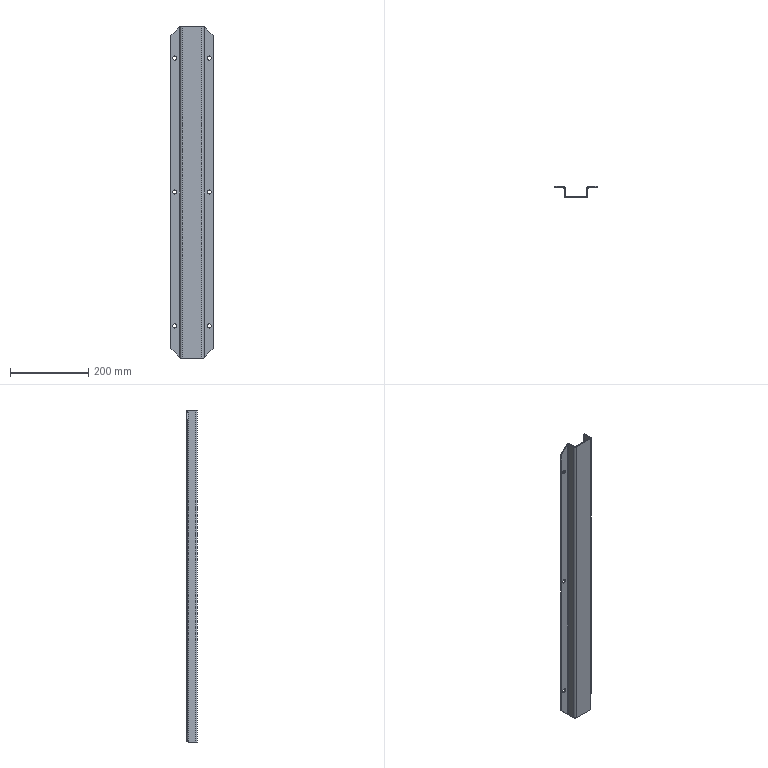Part | STEP file | 750078193 | 1 solid | 42 faces | box 108 x 27.5 x 850 mm | volume 319697 mm3 | cylinder 20 | plane 18 | spline 4 | commonest cylinder face diameters 10.5 x12 4 x4 9 x4
STEP:
#1=CARTESIAN_POINT('',(44.,27.5,-5.25));
#2=VERTEX_POINT('',#1);
#3=CARTESIAN_POINT('',(44.,27.5,5.25));
#4=VERTEX_POINT('',#3);
#5=CARTESIAN_POINT('',(44.,27.5,0.));
#6=DIRECTION('',(0.,1.,0.));
#7=DIRECTION('',(0.,0.,-1.));
#8=AXIS2_PLACEMENT_3D('',#5,#6,#7);
#9=CIRCLE('',#8,5.25);
#10=EDGE_CURVE('',#2,#4,#9,.T.);
#11=ORIENTED_EDGE('',*,*,#10,.T.);
#12=CARTESIAN_POINT('',(44.,25.,5.25));
#13=VERTEX_POINT('',#12);
#14=CARTESIAN_POINT('',(44.,882.275,5.25));
#15=DIRECTION('',(0.,-1.,0.));
#16=VECTOR('',#15,1000.);
#17=LINE('',#14,#16);
#18=EDGE_CURVE('',#4,#13,#17,.T.);
#19=ORIENTED_EDGE('',*,*,#18,.T.);
#20=CARTESIAN_POINT('',(44.,25.,-5.25));
#21=VERTEX_POINT('',#20);
#22=CARTESIAN_POINT('',(44.,25.,0.));
#23=DIRECTION('',(0.,1.,0.));
#24=DIRECTION('',(0.,0.,-1.));
#25=AXIS2_PLACEMENT_3D('',#22,#23,#24);
#26=CIRCLE('',#25,5.25);
#27=EDGE_CURVE('',#21,#13,#26,.T.);
#28=ORIENTED_EDGE('',*,*,#27,.F.);
#29=CARTESIAN_POINT('',(44.,882.275,-5.25));
#30=DIRECTION('',(0.,-1.,0.));
#31=VECTOR('',#30,1000.);
#32=LINE('',#29,#31);
#33=EDGE_CURVE('',#2,#21,#32,.T.);
#34=ORIENTED_EDGE('',*,*,#33,.F.);
#35=EDGE_LOOP('',(#11,#19,#28,#34));
#36=FACE_OUTER_BOUND('',#35,.T.);
#37=CARTESIAN_POINT('',(44.,882.275,0.));
#38=DIRECTION('',(0.,-1.,0.));
#39=DIRECTION('',(0.,0.,-1.));
#40=AXIS2_PLACEMENT_3D('',#37,#38,#39);
#41=CYLINDRICAL_SURFACE('',#40,5.25);
#42=ADVANCED_FACE('',(#36),#41,.F.);
#43=CARTESIAN_POINT('',(44.,27.5,-348.25));
#44=VERTEX_POINT('',#43);
#45=CARTESIAN_POINT('',(44.,27.5,-337.75));
#46=VERTEX_POINT('',#45);
#47=CARTESIAN_POINT('',(44.,27.5,-343.));
#48=DIRECTION('',(0.,1.,0.));
#49=DIRECTION('',(0.,0.,-1.));
#50=AXIS2_PLACEMENT_3D('',#47,#48,#49);
#51=CIRCLE('',#50,5.25);
#52=EDGE_CURVE('',#44,#46,#51,.T.);
#53=ORIENTED_EDGE('',*,*,#52,.T.);
#54=CARTESIAN_POINT('',(44.,25.,-337.75));
#55=VERTEX_POINT('',#54);
#56=CARTESIAN_POINT('',(44.,882.275,-337.75));
#57=DIRECTION('',(0.,-1.,0.));
#58=VECTOR('',#57,1000.);
#59=LINE('',#56,#58);
#60=EDGE_CURVE('',#46,#55,#59,.T.);
#61=ORIENTED_EDGE('',*,*,#60,.T.);
#62=CARTESIAN_POINT('',(44.,25.,-348.25));
#63=VERTEX_POINT('',#62);
#64=CARTESIAN_POINT('',(44.,25.,-343.));
#65=DIRECTION('',(0.,1.,0.));
#66=DIRECTION('',(0.,0.,-1.));
#67=AXIS2_PLACEMENT_3D('',#64,#65,#66);
#68=CIRCLE('',#67,5.25);
#69=EDGE_CURVE('',#63,#55,#68,.T.);
#70=ORIENTED_EDGE('',*,*,#69,.F.);
#71=CARTESIAN_POINT('',(44.,882.275,-348.25));
#72=DIRECTION('',(0.,-1.,0.));
#73=VECTOR('',#72,1000.);
#74=LINE('',#71,#73);
#75=EDGE_CURVE('',#44,#63,#74,.T.);
#76=ORIENTED_EDGE('',*,*,#75,.F.);
#77=EDGE_LOOP('',(#53,#61,#70,#76));
#78=FACE_OUTER_BOUND('',#77,.T.);
#79=CARTESIAN_POINT('',(44.,882.275,-343.));
#80=DIRECTION('',(0.,-1.,0.));
#81=DIRECTION('',(0.,0.,-1.));
#82=AXIS2_PLACEMENT_3D('',#79,#80,#81);
#83=CYLINDRICAL_SURFACE('',#82,5.25);
#84=ADVANCED_FACE('',(#78),#83,.F.);
#85=CARTESIAN_POINT('',(44.,27.5,337.75));
#86=VERTEX_POINT('',#85);
#87=CARTESIAN_POINT('',(44.,27.5,348.25));
#88=VERTEX_POINT('',#87);
#89=CARTESIAN_POINT('',(44.,27.5,343.));
#90=DIRECTION('',(0.,1.,0.));
#91=DIRECTION('',(0.,0.,-1.));
#92=AXIS2_PLACEMENT_3D('',#89,#90,#91);
#93=CIRCLE('',#92,5.25);
#94=EDGE_CURVE('',#86,#88,#93,.T.);
#95=ORIENTED_EDGE('',*,*,#94,.T.);
#96=CARTESIAN_POINT('',(44.,25.,348.25));
#97=VERTEX_POINT('',#96);
#98=CARTESIAN_POINT('',(44.,882.275,348.25));
#99=DIRECTION('',(0.,-1.,0.));
#100=VECTOR('',#99,1000.);
#101=LINE('',#98,#100);
#102=EDGE_CURVE('',#88,#97,#101,.T.);
#103=ORIENTED_EDGE('',*,*,#102,.T.);
#104=CARTESIAN_POINT('',(44.,25.,337.75));
#105=VERTEX_POINT('',#104);
#106=CARTESIAN_POINT('',(44.,25.,343.));
#107=DIRECTION('',(0.,1.,0.));
#108=DIRECTION('',(0.,0.,-1.));
#109=AXIS2_PLACEMENT_3D('',#106,#107,#108);
#110=CIRCLE('',#109,5.25);
#111=EDGE_CURVE('',#105,#97,#110,.T.);
#112=ORIENTED_EDGE('',*,*,#111,.F.);
#113=CARTESIAN_POINT('',(44.,882.275,337.75));
#114=DIRECTION('',(0.,-1.,0.));
#115=VECTOR('',#114,1000.);
#116=LINE('',#113,#115);
#117=EDGE_CURVE('',#86,#105,#116,.T.);
#118=ORIENTED_EDGE('',*,*,#117,.F.);
#119=EDGE_LOOP('',(#95,#103,#112,#118));
#120=FACE_OUTER_BOUND('',#119,.T.);
#121=CARTESIAN_POINT('',(44.,882.275,343.));
#122=DIRECTION('',(0.,-1.,0.));
#123=DIRECTION('',(0.,0.,-1.));
#124=AXIS2_PLACEMENT_3D('',#121,#122,#123);
#125=CYLINDRICAL_SURFACE('',#124,5.25);
#126=ADVANCED_FACE('',(#120),#125,.F.);
#127=CARTESIAN_POINT('',(-44.,27.5,337.75));
#128=VERTEX_POINT('',#127);
#129=CARTESIAN_POINT('',(-44.,27.5,348.25));
#130=VERTEX_POINT('',#129);
#131=CARTESIAN_POINT('',(-44.,27.5,343.));
#132=DIRECTION('',(0.,1.,0.));
#133=DIRECTION('',(0.,0.,-1.));
#134=AXIS2_PLACEMENT_3D('',#131,#132,#133);
#135=CIRCLE('',#134,5.25);
#136=EDGE_CURVE('',#128,#130,#135,.T.);
#137=ORIENTED_EDGE('',*,*,#136,.T.);
#138=CARTESIAN_POINT('',(-44.,25.,348.25));
#139=VERTEX_POINT('',#138);
#140=CARTESIAN_POINT('',(-44.,882.275,348.25));
#141=DIRECTION('',(0.,-1.,0.));
#142=VECTOR('',#141,1000.);
#143=LINE('',#140,#142);
#144=EDGE_CURVE('',#130,#139,#143,.T.);
#145=ORIENTED_EDGE('',*,*,#144,.T.);
#146=CARTESIAN_POINT('',(-44.,25.,337.75));
#147=VERTEX_POINT('',#146);
#148=CARTESIAN_POINT('',(-44.,25.,343.));
#149=DIRECTION('',(0.,1.,0.));
#150=DIRECTION('',(0.,0.,-1.));
#151=AXIS2_PLACEMENT_3D('',#148,#149,#150);
#152=CIRCLE('',#151,5.25);
#153=EDGE_CURVE('',#147,#139,#152,.T.);
#154=ORIENTED_EDGE('',*,*,#153,.F.);
#155=CARTESIAN_POINT('',(-44.,882.275,337.75));
#156=DIRECTION('',(0.,-1.,0.));
#157=VECTOR('',#156,1000.);
#158=LINE('',#155,#157);
#159=EDGE_CURVE('',#128,#147,#158,.T.);
#160=ORIENTED_EDGE('',*,*,#159,.F.);
#161=EDGE_LOOP('',(#137,#145,#154,#160));
#162=FACE_OUTER_BOUND('',#161,.T.);
#163=CARTESIAN_POINT('',(-44.,882.275,343.));
#164=DIRECTION('',(0.,-1.,0.));
#165=DIRECTION('',(0.,0.,-1.));
#166=AXIS2_PLACEMENT_3D('',#163,#164,#165);
#167=CYLINDRICAL_SURFACE('',#166,5.25);
#168=ADVANCED_FACE('',(#162),#167,.F.);
#169=CARTESIAN_POINT('',(-44.,27.5,-348.25));
#170=VERTEX_POINT('',#169);
#171=CARTESIAN_POINT('',(-44.,27.5,-337.75));
#172=VERTEX_POINT('',#171);
#173=CARTESIAN_POINT('',(-44.,27.5,-343.));
#174=DIRECTION('',(0.,1.,0.));
#175=DIRECTION('',(0.,0.,-1.));
#176=AXIS2_PLACEMENT_3D('',#173,#174,#175);
#177=CIRCLE('',#176,5.25);
#178=EDGE_CURVE('',#170,#172,#177,.T.);
#179=ORIENTED_EDGE('',*,*,#178,.T.);
#180=CARTESIAN_POINT('',(-44.,25.,-337.75));
#181=VERTEX_POINT('',#180);
#182=CARTESIAN_POINT('',(-44.,882.275,-337.75));
#183=DIRECTION('',(0.,-1.,0.));
#184=VECTOR('',#183,1000.);
#185=LINE('',#182,#184);
#186=EDGE_CURVE('',#172,#181,#185,.T.);
#187=ORIENTED_EDGE('',*,*,#186,.T.);
#188=CARTESIAN_POINT('',(-44.,25.,-348.25));
#189=VERTEX_POINT('',#188);
#190=CARTESIAN_POINT('',(-44.,25.,-343.));
#191=DIRECTION('',(0.,1.,0.));
#192=DIRECTION('',(0.,0.,-1.));
#193=AXIS2_PLACEMENT_3D('',#190,#191,#192);
#194=CIRCLE('',#193,5.25);
#195=EDGE_CURVE('',#189,#181,#194,.T.);
#196=ORIENTED_EDGE('',*,*,#195,.F.);
#197=CARTESIAN_POINT('',(-44.,882.275,-348.25));
#198=DIRECTION('',(0.,-1.,0.));
#199=VECTOR('',#198,1000.);
#200=LINE('',#197,#199);
#201=EDGE_CURVE('',#170,#189,#200,.T.);
#202=ORIENTED_EDGE('',*,*,#201,.F.);
#203=EDGE_LOOP('',(#179,#187,#196,#202));
#204=FACE_OUTER_BOUND('',#203,.T.);
#205=CARTESIAN_POINT('',(-44.,882.275,-343.));
#206=DIRECTION('',(0.,-1.,0.));
#207=DIRECTION('',(0.,0.,-1.));
#208=AXIS2_PLACEMENT_3D('',#205,#206,#207);
#209=CYLINDRICAL_SURFACE('',#208,5.25);
#210=ADVANCED_FACE('',(#204),#209,.F.);
#211=CARTESIAN_POINT('',(-44.,27.5,-5.25));
#212=VERTEX_POINT('',#211);
#213=CARTESIAN_POINT('',(-44.,27.5,5.25));
#214=VERTEX_POINT('',#213);
#215=CARTESIAN_POINT('',(-44.,27.5,0.));
#216=DIRECTION('',(0.,1.,0.));
#217=DIRECTION('',(0.,0.,-1.));
#218=AXIS2_PLACEMENT_3D('',#215,#216,#217);
#219=CIRCLE('',#218,5.25);
#220=EDGE_CURVE('',#212,#214,#219,.T.);
#221=ORIENTED_EDGE('',*,*,#220,.T.);
#222=CARTESIAN_POINT('',(-44.,25.,5.25));
#223=VERTEX_POINT('',#222);
#224=CARTESIAN_POINT('',(-44.,882.275,5.25));
#225=DIRECTION('',(0.,-1.,0.));
#226=VECTOR('',#225,1000.);
#227=LINE('',#224,#226);
#228=EDGE_CURVE('',#214,#223,#227,.T.);
#229=ORIENTED_EDGE('',*,*,#228,.T.);
#230=CARTESIAN_POINT('',(-44.,25.,-5.25));
#231=VERTEX_POINT('',#230);
#232=CARTESIAN_POINT('',(-44.,25.,0.));
#233=DIRECTION('',(0.,1.,0.));
#234=DIRECTION('',(0.,0.,-1.));
#235=AXIS2_PLACEMENT_3D('',#232,#233,#234);
#236=CIRCLE('',#235,5.25);
#237=EDGE_CURVE('',#231,#223,#236,.T.);
#238=ORIENTED_EDGE('',*,*,#237,.F.);
#239=CARTESIAN_POINT('',(-44.,882.275,-5.25));
#240=DIRECTION('',(0.,-1.,0.));
#241=VECTOR('',#240,1000.);
#242=LINE('',#239,#241);
#243=EDGE_CURVE('',#212,#231,#242,.T.);
#244=ORIENTED_EDGE('',*,*,#243,.F.);
#245=EDGE_LOOP('',(#221,#229,#238,#244));
#246=FACE_OUTER_BOUND('',#245,.T.);
#247=CARTESIAN_POINT('',(-44.,882.275,0.));
#248=DIRECTION('',(0.,-1.,0.));
#249=DIRECTION('',(0.,0.,-1.));
#250=AXIS2_PLACEMENT_3D('',#247,#248,#249);
#251=CYLINDRICAL_SURFACE('',#250,5.25);
#252=ADVANCED_FACE('',(#246),#251,.F.);
#253=CARTESIAN_POINT('',(-25.5,2.5,425.));
#254=VERTEX_POINT('',#253);
#255=CARTESIAN_POINT('',(-25.5,2.5,-425.));
#256=VERTEX_POINT('',#255);
#257=CARTESIAN_POINT('',(-25.5,2.5,425.));
#258=DIRECTION('',(0.,0.,-1.));
#259=VECTOR('',#258,1000.);
#260=LINE('',#257,#259);
#261=EDGE_CURVE('',#254,#256,#260,.T.);
#262=ORIENTED_EDGE('',*,*,#261,.F.);
#263=CARTESIAN_POINT('',(25.5,2.5,425.));
#264=VERTEX_POINT('',#263);
#265=CARTESIAN_POINT('',(30.,2.5,425.));
#266=DIRECTION('',(-1.,0.,0.));
#267=VECTOR('',#266,1000.);
#268=LINE('',#265,#267);
#269=EDGE_CURVE('',#264,#254,#268,.T.);
#270=ORIENTED_EDGE('',*,*,#269,.F.);
#271=CARTESIAN_POINT('',(25.5,2.5,-425.));
#272=VERTEX_POINT('',#271);
#273=CARTESIAN_POINT('',(25.5,2.5,425.));
#274=DIRECTION('',(0.,0.,1.));
#275=VECTOR('',#274,1000.);
#276=LINE('',#273,#275);
#277=EDGE_CURVE('',#272,#264,#276,.T.);
#278=ORIENTED_EDGE('',*,*,#277,.F.);
#279=CARTESIAN_POINT('',(30.,2.5,-425.));
#280=DIRECTION('',(1.,0.,0.));
#281=VECTOR('',#280,1000.);
#282=LINE('',#279,#281);
#283=EDGE_CURVE('',#256,#272,#282,.T.);
#284=ORIENTED_EDGE('',*,*,#283,.F.);
#285=EDGE_LOOP('',(#262,#270,#278,#284));
#286=FACE_OUTER_BOUND('',#285,.T.);
#287=CARTESIAN_POINT('',(30.,2.5,425.));
#288=DIRECTION('',(0.,-1.,0.));
#289=DIRECTION('',(1.,0.,0.));
#290=AXIS2_PLACEMENT_3D('',#287,#288,#289);
#291=PLANE('',#290);
#292=ADVANCED_FACE('',(#286),#291,.F.);
#293=CARTESIAN_POINT('',(30.,23.,-425.));
#294=VERTEX_POINT('',#293);
#295=CARTESIAN_POINT('',(27.5,23.,-425.));
#296=VERTEX_POINT('',#295);
#297=CARTESIAN_POINT('',(54.,23.,-425.));
#298=DIRECTION('',(-1.,0.,0.));
#299=VECTOR('',#298,1000.);
#300=LINE('',#297,#299);
#301=EDGE_CURVE('',#294,#296,#300,.T.);
#302=ORIENTED_EDGE('',*,*,#301,.F.);
#303=CARTESIAN_POINT('',(30.,4.5,-425.));
#304=VERTEX_POINT('',#303);
#305=CARTESIAN_POINT('',(30.,25.,-425.));
#306=DIRECTION('',(0.,1.,0.));
#307=VECTOR('',#306,1000.);
#308=LINE('',#305,#307);
#309=EDGE_CURVE('',#304,#294,#308,.T.);
#310=ORIENTED_EDGE('',*,*,#309,.F.);
#311=CARTESIAN_POINT('',(25.5,0.,-425.));
#312=VERTEX_POINT('',#311);
#313=CARTESIAN_POINT('',(25.5,4.5,-425.));
#314=DIRECTION('',(0.,0.,1.));
#315=DIRECTION('',(-1.,0.,0.));
#316=AXIS2_PLACEMENT_3D('',#313,#314,#315);
#317=CIRCLE('',#316,4.5);
#318=EDGE_CURVE('',#312,#304,#317,.T.);
#319=ORIENTED_EDGE('',*,*,#318,.F.);
#320=CARTESIAN_POINT('',(-25.5,0.,-425.));
#321=VERTEX_POINT('',#320);
#322=CARTESIAN_POINT('',(54.,0.,-425.));
#323=DIRECTION('',(1.,0.,0.));
#324=VECTOR('',#323,1000.);
#325=LINE('',#322,#324);
#326=EDGE_CURVE('',#321,#312,#325,.T.);
#327=ORIENTED_EDGE('',*,*,#326,.F.);
#328=CARTESIAN_POINT('',(-30.,4.5,-425.));
#329=VERTEX_POINT('',#328);
#330=CARTESIAN_POINT('',(-25.5,4.5,-425.));
#331=DIRECTION('',(0.,0.,1.));
#332=DIRECTION('',(-1.,0.,0.));
#333=AXIS2_PLACEMENT_3D('',#330,#331,#332);
#334=CIRCLE('',#333,4.5);
#335=EDGE_CURVE('',#329,#321,#334,.T.);
#336=ORIENTED_EDGE('',*,*,#335,.F.);
#337=CARTESIAN_POINT('',(-30.,23.,-425.));
#338=VERTEX_POINT('',#337);
#339=CARTESIAN_POINT('',(-30.,25.,-425.));
#340=DIRECTION('',(0.,-1.,0.));
#341=VECTOR('',#340,1000.);
#342=LINE('',#339,#341);
#343=EDGE_CURVE('',#338,#329,#342,.T.);
#344=ORIENTED_EDGE('',*,*,#343,.F.);
#345=CARTESIAN_POINT('',(-27.5,23.,-425.));
#346=VERTEX_POINT('',#345);
#347=CARTESIAN_POINT('',(54.,23.,-425.));
#348=DIRECTION('',(-1.,0.,0.));
#349=VECTOR('',#348,1000.);
#350=LINE('',#347,#349);
#351=EDGE_CURVE('',#346,#338,#350,.T.);
#352=ORIENTED_EDGE('',*,*,#351,.F.);
#353=CARTESIAN_POINT('',(-27.5,4.5,-425.));
#354=VERTEX_POINT('',#353);
#355=CARTESIAN_POINT('',(-27.5,25.,-425.));
#356=DIRECTION('',(0.,1.,0.));
#357=VECTOR('',#356,1000.);
#358=LINE('',#355,#357);
#359=EDGE_CURVE('',#354,#346,#358,.T.);
#360=ORIENTED_EDGE('',*,*,#359,.F.);
#361=CARTESIAN_POINT('',(-25.5,4.5,-425.));
#362=DIRECTION('',(0.,0.,-1.));
#363=DIRECTION('',(-1.,0.,0.));
#364=AXIS2_PLACEMENT_3D('',#361,#362,#363);
#365=CIRCLE('',#364,2.);
#366=EDGE_CURVE('',#256,#354,#365,.T.);
#367=ORIENTED_EDGE('',*,*,#366,.F.);
#368=ORIENTED_EDGE('',*,*,#283,.T.);
#369=CARTESIAN_POINT('',(27.5,4.5,-425.));
#370=VERTEX_POINT('',#369);
#371=CARTESIAN_POINT('',(25.5,4.5,-425.));
#372=DIRECTION('',(0.,0.,-1.));
#373=DIRECTION('',(-1.,0.,0.));
#374=AXIS2_PLACEMENT_3D('',#371,#372,#373);
#375=CIRCLE('',#374,2.);
#376=EDGE_CURVE('',#370,#272,#375,.T.);
#377=ORIENTED_EDGE('',*,*,#376,.F.);
#378=CARTESIAN_POINT('',(27.5,25.,-425.));
#379=DIRECTION('',(0.,-1.,0.));
#380=VECTOR('',#379,1000.);
#381=LINE('',#378,#380);
#382=EDGE_CURVE('',#296,#370,#381,.T.);
#383=ORIENTED_EDGE('',*,*,#382,.F.);
#384=EDGE_LOOP('',(#302,#310,#319,#327,#336,#344,#352,#360,#367,#368,#377,#383));
#385=FACE_OUTER_BOUND('',#384,.T.);
#386=CARTESIAN_POINT('',(54.,25.,-425.));
#387=DIRECTION('',(0.,0.,1.));
#388=DIRECTION('',(1.,0.,0.));
#389=AXIS2_PLACEMENT_3D('',#386,#387,#388);
#390=PLANE('',#389);
#391=ADVANCED_FACE('',(#385),#390,.F.);
#392=CARTESIAN_POINT('',(-27.5,4.5,425.));
#393=VERTEX_POINT('',#392);
#394=CARTESIAN_POINT('',(-27.5,4.5,425.));
#395=DIRECTION('',(0.,0.,-1.));
#396=VECTOR('',#395,1000.);
#397=LINE('',#394,#396);
#398=EDGE_CURVE('',#393,#354,#397,.T.);
#399=ORIENTED_EDGE('',*,*,#398,.F.);
#400=CARTESIAN_POINT('',(-25.5,4.5,425.));
#401=DIRECTION('',(0.,0.,-1.));
#402=DIRECTION('',(-1.,0.,0.));
#403=AXIS2_PLACEMENT_3D('',#400,#401,#402);
#404=CIRCLE('',#403,2.);
#405=EDGE_CURVE('',#254,#393,#404,.T.);
#406=ORIENTED_EDGE('',*,*,#405,.F.);
#407=ORIENTED_EDGE('',*,*,#261,.T.);
#408=ORIENTED_EDGE('',*,*,#366,.T.);
#409=EDGE_LOOP('',(#399,#406,#407,#408));
#410=FACE_OUTER_BOUND('',#409,.T.);
#411=CARTESIAN_POINT('',(-25.5,4.5,425.));
#412=DIRECTION('',(0.,0.,-1.));
#413=DIRECTION('',(-1.,0.,0.));
#414=AXIS2_PLACEMENT_3D('',#411,#412,#413);
#415=CYLINDRICAL_SURFACE('',#414,2.);
#416=ADVANCED_FACE('',(#410),#415,.F.);
#417=CARTESIAN_POINT('',(25.5,0.,425.));
#418=VERTEX_POINT('',#417);
#419=CARTESIAN_POINT('',(30.,4.5,425.));
#420=VERTEX_POINT('',#419);
#421=CARTESIAN_POINT('',(25.5,4.5,425.));
#422=DIRECTION('',(0.,0.,1.));
#423=DIRECTION('',(-1.,0.,0.));
#424=AXIS2_PLACEMENT_3D('',#421,#422,#423);
#425=CIRCLE('',#424,4.5);
#426=EDGE_CURVE('',#418,#420,#425,.T.);
#427=ORIENTED_EDGE('',*,*,#426,.T.);
#428=CARTESIAN_POINT('',(30.,23.,425.));
#429=VERTEX_POINT('',#428);
#430=CARTESIAN_POINT('',(30.,25.,425.));
#431=DIRECTION('',(0.,1.,0.));
#432=VECTOR('',#431,1000.);
#433=LINE('',#430,#432);
#434=EDGE_CURVE('',#420,#429,#433,.T.);
#435=ORIENTED_EDGE('',*,*,#434,.T.);
#436=CARTESIAN_POINT('',(27.5,23.,425.));
#437=VERTEX_POINT('',#436);
#438=CARTESIAN_POINT('',(-30.,23.,425.));
#439=DIRECTION('',(-1.,0.,0.));
#440=VECTOR('',#439,1000.);
#441=LINE('',#438,#440);
#442=EDGE_CURVE('',#429,#437,#441,.T.);
#443=ORIENTED_EDGE('',*,*,#442,.T.);
#444=CARTESIAN_POINT('',(27.5,4.5,425.));
#445=VERTEX_POINT('',#444);
#446=CARTESIAN_POINT('',(27.5,25.,425.));
#447=DIRECTION('',(0.,-1.,0.));
#448=VECTOR('',#447,1000.);
#449=LINE('',#446,#448);
#450=EDGE_CURVE('',#437,#445,#449,.T.);
#451=ORIENTED_EDGE('',*,*,#450,.T.);
#452=CARTESIAN_POINT('',(25.5,4.5,425.));
#453=DIRECTION('',(0.,0.,-1.));
#454=DIRECTION('',(-1.,0.,0.));
#455=AXIS2_PLACEMENT_3D('',#452,#453,#454);
#456=CIRCLE('',#455,2.);
#457=EDGE_CURVE('',#445,#264,#456,.T.);
#458=ORIENTED_EDGE('',*,*,#457,.T.);
#459=ORIENTED_EDGE('',*,*,#269,.T.);
#460=ORIENTED_EDGE('',*,*,#405,.T.);
#461=CARTESIAN_POINT('',(-27.5,23.,425.));
#462=VERTEX_POINT('',#461);
#463=CARTESIAN_POINT('',(-27.5,25.,425.));
#464=DIRECTION('',(0.,1.,0.));
#465=VECTOR('',#464,1000.);
#466=LINE('',#463,#465);
#467=EDGE_CURVE('',#393,#462,#466,.T.);
#468=ORIENTED_EDGE('',*,*,#467,.T.);
#469=CARTESIAN_POINT('',(-30.,23.,425.));
#470=VERTEX_POINT('',#469);
#471=CARTESIAN_POINT('',(-30.,23.,425.));
#472=DIRECTION('',(-1.,0.,0.));
#473=VECTOR('',#472,1000.);
#474=LINE('',#471,#473);
#475=EDGE_CURVE('',#462,#470,#474,.T.);
#476=ORIENTED_EDGE('',*,*,#475,.T.);
#477=CARTESIAN_POINT('',(-30.,4.5,425.));
#478=VERTEX_POINT('',#477);
#479=CARTESIAN_POINT('',(-30.,25.,425.));
#480=DIRECTION('',(0.,-1.,0.));
#481=VECTOR('',#480,1000.);
#482=LINE('',#479,#481);
#483=EDGE_CURVE('',#470,#478,#482,.T.);
#484=ORIENTED_EDGE('',*,*,#483,.T.);
#485=CARTESIAN_POINT('',(-25.5,0.,425.));
#486=VERTEX_POINT('',#485);
#487=CARTESIAN_POINT('',(-25.5,4.5,425.));
#488=DIRECTION('',(0.,0.,1.));
#489=DIRECTION('',(-1.,0.,0.));
#490=AXIS2_PLACEMENT_3D('',#487,#488,#489);
#491=CIRCLE('',#490,4.5);
#492=EDGE_CURVE('',#478,#486,#491,.T.);
#493=ORIENTED_EDGE('',*,*,#492,.T.);
#494=CARTESIAN_POINT('',(-30.,0.,425.));
#495=DIRECTION('',(1.,0.,0.));
#496=VECTOR('',#495,1000.);
#497=LINE('',#494,#496);
#498=EDGE_CURVE('',#486,#418,#497,.T.);
#499=ORIENTED_EDGE('',*,*,#498,.T.);
#500=EDGE_LOOP('',(#427,#435,#443,#451,#458,#459,#460,#468,#476,#484,#493,#499));
#501=FACE_OUTER_BOUND('',#500,.T.);
#502=CARTESIAN_POINT('',(-30.,25.,425.));
#503=DIRECTION('',(0.,0.,1.));
#504=DIRECTION('',(1.,0.,0.));
#505=AXIS2_PLACEMENT_3D('',#502,#503,#504);
#506=PLANE('',#505);
#507=ADVANCED_FACE('',(#501),#506,.T.);
#508=ORIENTED_EDGE('',*,*,#277,.T.);
#509=ORIENTED_EDGE('',*,*,#457,.F.);
#510=CARTESIAN_POINT('',(27.5,4.5,425.));
#511=DIRECTION('',(0.,0.,1.));
#512=VECTOR('',#511,1000.);
#513=LINE('',#510,#512);
#514=EDGE_CURVE('',#370,#445,#513,.T.);
#515=ORIENTED_EDGE('',*,*,#514,.F.);
#516=ORIENTED_EDGE('',*,*,#376,.T.);
#517=EDGE_LOOP('',(#508,#509,#515,#516));
#518=FACE_OUTER_BOUND('',#517,.T.);
#519=CARTESIAN_POINT('',(25.5,4.5,425.));
#520=DIRECTION('',(0.,0.,-1.));
#521=DIRECTION('',(-1.,0.,0.));
#522=AXIS2_PLACEMENT_3D('',#519,#520,#521);
#523=CYLINDRICAL_SURFACE('',#522,2.);
#524=ADVANCED_FACE('',(#518),#523,.F.);
#525=ORIENTED_EDGE('',*,*,#514,.T.);
#526=ORIENTED_EDGE('',*,*,#450,.F.);
#527=CARTESIAN_POINT('',(27.5,23.,425.));
#528=DIRECTION('',(0.,0.,1.));
#529=VECTOR('',#528,1000.);
#530=LINE('',#527,#529);
#531=EDGE_CURVE('',#296,#437,#530,.T.);
#532=ORIENTED_EDGE('',*,*,#531,.F.);
#533=ORIENTED_EDGE('',*,*,#382,.T.);
#534=EDGE_LOOP('',(#525,#526,#532,#533));
#535=FACE_OUTER_BOUND('',#534,.T.);
#536=CARTESIAN_POINT('',(27.5,25.,425.));
#537=DIRECTION('',(1.,0.,0.));
#538=DIRECTION('',(0.,1.,0.));
#539=AXIS2_PLACEMENT_3D('',#536,#537,#538);
#540=PLANE('',#539);
#541=ADVANCED_FACE('',(#535),#540,.F.);
#542=ORIENTED_EDGE('',*,*,#301,.T.);
#543=CARTESIAN_POINT('',(32.,27.5,-423.));
#544=VERTEX_POINT('',#543);
#545=CARTESIAN_POINT('',(27.5,23.,-425.));
#546=CARTESIAN_POINT('',(27.5,25.25,-425.));
#547=CARTESIAN_POINT('',(29.,27.5,-424.333));
#548=CARTESIAN_POINT('',(32.,27.5,-423.));
#549=(BOUNDED_CURVE()B_SPLINE_CURVE(3,(#545,#546,#547,#548),.UNSPECIFIED.,.F.,.F.)B_SPLINE_CURVE_WITH_KNOTS((4,4),(0.,0.007455),.UNSPECIFIED.)CURVE()GEOMETRIC_REPRESENTATION_ITEM()RATIONAL_B_SPLINE_CURVE((1.,0.6667,0.5,0.5))REPRESENTATION_ITEM(''));
#550=EDGE_CURVE('',#296,#544,#549,.T.);
#551=ORIENTED_EDGE('',*,*,#550,.T.);
#552=CARTESIAN_POINT('',(32.,25.,-423.));
#553=VERTEX_POINT('',#552);
#554=CARTESIAN_POINT('',(32.,26.25,-423.));
#555=DIRECTION('',(0.,-1.,0.));
#556=VECTOR('',#555,1000.);
#557=LINE('',#554,#556);
#558=EDGE_CURVE('',#544,#553,#557,.T.);
#559=ORIENTED_EDGE('',*,*,#558,.T.);
#560=CARTESIAN_POINT('',(32.,25.,-423.));
#561=CARTESIAN_POINT('',(30.667,25.,-424.333));
#562=CARTESIAN_POINT('',(30.,24.,-425.));
#563=CARTESIAN_POINT('',(30.,23.,-425.));
#564=(BOUNDED_CURVE()B_SPLINE_CURVE(3,(#560,#561,#562,#563),.UNSPECIFIED.,.F.,.F.)B_SPLINE_CURVE_WITH_KNOTS((4,4),(0.,0.003785),.UNSPECIFIED.)CURVE()GEOMETRIC_REPRESENTATION_ITEM()RATIONAL_B_SPLINE_CURVE((0.5,0.5,0.6667,1.))REPRESENTATION_ITEM(''));
#565=EDGE_CURVE('',#553,#294,#564,.T.);
#566=ORIENTED_EDGE('',*,*,#565,.T.);
#567=EDGE_LOOP('',(#542,#551,#559,#566));
#568=FACE_OUTER_BOUND('',#567,.T.);
#569=CARTESIAN_POINT('',(30.,23.,-425.));
#570=CARTESIAN_POINT('',(29.167,23.,-425.));
#571=CARTESIAN_POINT('',(28.333,23.,-425.));
#572=CARTESIAN_POINT('',(27.5,23.,-425.));
#573=CARTESIAN_POINT('',(30.,19.,-425.));
#574=CARTESIAN_POINT('',(29.167,17.333,-425.));
#575=CARTESIAN_POINT('',(28.333,15.667,-425.));
#576=CARTESIAN_POINT('',(27.5,14.,-425.));
#577=CARTESIAN_POINT('',(34.,19.,-421.));
#578=CARTESIAN_POINT('',(34.833,17.333,-421.));
#579=CARTESIAN_POINT('',(35.667,15.667,-421.));
#580=CARTESIAN_POINT('',(36.5,14.,-421.));
#581=CARTESIAN_POINT('',(34.,23.,-421.));
#582=CARTESIAN_POINT('',(34.833,23.,-421.));
#583=CARTESIAN_POINT('',(35.667,23.,-421.));
#584=CARTESIAN_POINT('',(36.5,23.,-421.));
#585=CARTESIAN_POINT('',(34.,27.,-421.));
#586=CARTESIAN_POINT('',(34.833,28.667,-421.));
#587=CARTESIAN_POINT('',(35.667,30.333,-421.));
#588=CARTESIAN_POINT('',(36.5,32.,-421.));
#589=CARTESIAN_POINT('',(30.,27.,-425.));
#590=CARTESIAN_POINT('',(29.167,28.667,-425.));
#591=CARTESIAN_POINT('',(28.333,30.333,-425.));
#592=CARTESIAN_POINT('',(27.5,32.,-425.));
#593=CARTESIAN_POINT('',(30.,23.,-425.));
#594=CARTESIAN_POINT('',(29.167,23.,-425.));
#595=CARTESIAN_POINT('',(28.333,23.,-425.));
#596=CARTESIAN_POINT('',(27.5,23.,-425.));
#597=(BOUNDED_SURFACE()B_SPLINE_SURFACE(3,3,((#569,#570,#571,#572),(#573,#574,#575,#576),(#577,#578,#579,#580),(#581,#582,#583,#584),(#585,#586,#587,#588),(#589,#590,#591,#592),(#593,#594,#595,#596)),.UNSPECIFIED.,.T.,.F.,.F.)B_SPLINE_SURFACE_WITH_KNOTS((4,3,4),(4,4),(0.,0.5,1.),(0.,1.),.UNSPECIFIED.)GEOMETRIC_REPRESENTATION_ITEM()RATIONAL_B_SPLINE_SURFACE(((1.,1.,1.,1.),(0.3333,0.3333,0.3333,0.3333),(0.3333,0.3333,0.3333,0.3333),(1.,1.,1.,1.),(0.3333,0.3333,0.3333,0.3333),(0.3333,0.3333,0.3333,0.3333),(1.,1.,1.,1.)))REPRESENTATION_ITEM('')SURFACE());
#598=ADVANCED_FACE('',(#568),#597,.T.);
#599=ORIENTED_EDGE('',*,*,#434,.F.);
#600=CARTESIAN_POINT('',(30.,4.5,425.));
#601=DIRECTION('',(0.,0.,-1.));
#602=VECTOR('',#601,1000.);
#603=LINE('',#600,#602);
#604=EDGE_CURVE('',#420,#304,#603,.T.);
#605=ORIENTED_EDGE('',*,*,#604,.T.);
#606=ORIENTED_EDGE('',*,*,#309,.T.);
#607=CARTESIAN_POINT('',(30.,23.,425.));
#608=DIRECTION('',(0.,0.,1.));
#609=VECTOR('',#608,1000.);
#610=LINE('',#607,#609);
#611=EDGE_CURVE('',#294,#429,#610,.T.);
#612=ORIENTED_EDGE('',*,*,#611,.T.);
#613=EDGE_LOOP('',(#599,#605,#606,#612));
#614=FACE_OUTER_BOUND('',#613,.T.);
#615=CARTESIAN_POINT('',(30.,25.,425.));
#616=DIRECTION('',(1.,0.,0.));
#617=DIRECTION('',(0.,1.,0.));
#618=AXIS2_PLACEMENT_3D('',#615,#616,#617);
#619=PLANE('',#618);
#620=ADVANCED_FACE('',(#614),#619,.T.);
#621=ORIENTED_EDGE('',*,*,#426,.F.);
#622=CARTESIAN_POINT('',(25.5,0.,425.));
#623=DIRECTION('',(0.,0.,-1.));
#624=VECTOR('',#623,1000.);
#625=LINE('',#622,#624);
#626=EDGE_CURVE('',#418,#312,#625,.T.);
#627=ORIENTED_EDGE('',*,*,#626,.T.);
#628=ORIENTED_EDGE('',*,*,#318,.T.);
#629=ORIENTED_EDGE('',*,*,#604,.F.);
#630=EDGE_LOOP('',(#621,#627,#628,#629));
#631=FACE_OUTER_BOUND('',#630,.T.);
#632=CARTESIAN_POINT('',(25.5,4.5,425.));
#633=DIRECTION('',(0.,0.,-1.));
#634=DIRECTION('',(-1.,0.,0.));
#635=AXIS2_PLACEMENT_3D('',#632,#633,#634);
#636=CYLINDRICAL_SURFACE('',#635,4.5);
#637=ADVANCED_FACE('',(#631),#636,.T.);
#638=ORIENTED_EDGE('',*,*,#498,.F.);
#639=CARTESIAN_POINT('',(-25.5,0.,425.));
#640=DIRECTION('',(0.,0.,-1.));
#641=VECTOR('',#640,1000.);
#642=LINE('',#639,#641);
#643=EDGE_CURVE('',#486,#321,#642,.T.);
#644=ORIENTED_EDGE('',*,*,#643,.T.);
#645=ORIENTED_EDGE('',*,*,#326,.T.);
#646=ORIENTED_EDGE('',*,*,#626,.F.);
#647=EDGE_LOOP('',(#638,#644,#645,#646));
#648=FACE_OUTER_BOUND('',#647,.T.);
#649=CARTESIAN_POINT('',(30.,0.,425.));
#650=DIRECTION('',(0.,-1.,0.));
#651=DIRECTION('',(1.,0.,0.));
#652=AXIS2_PLACEMENT_3D('',#649,#650,#651);
#653=PLANE('',#652);
#654=ADVANCED_FACE('',(#648),#653,.T.);
#655=ORIENTED_EDGE('',*,*,#492,.F.);
#656=CARTESIAN_POINT('',(-30.,4.5,425.));
#657=DIRECTION('',(0.,0.,-1.));
#658=VECTOR('',#657,1000.);
#659=LINE('',#656,#658);
#660=EDGE_CURVE('',#478,#329,#659,.T.);
#661=ORIENTED_EDGE('',*,*,#660,.T.);
#662=ORIENTED_EDGE('',*,*,#335,.T.);
#663=ORIENTED_EDGE('',*,*,#643,.F.);
#664=EDGE_LOOP('',(#655,#661,#662,#663));
#665=FACE_OUTER_BOUND('',#664,.T.);
#666=CARTESIAN_POINT('',(-25.5,4.5,425.));
#667=DIRECTION('',(0.,0.,-1.));
#668=DIRECTION('',(-1.,0.,0.));
#669=AXIS2_PLACEMENT_3D('',#666,#667,#668);
#670=CYLINDRICAL_SURFACE('',#669,4.5);
#671=ADVANCED_FACE('',(#665),#670,.T.);
#672=ORIENTED_EDGE('',*,*,#483,.F.);
#673=CARTESIAN_POINT('',(-30.,23.,425.));
#674=DIRECTION('',(0.,0.,-1.));
#675=VECTOR('',#674,1000.);
#676=LINE('',#673,#675);
#677=EDGE_CURVE('',#470,#338,#676,.T.);
#678=ORIENTED_EDGE('',*,*,#677,.T.);
#679=ORIENTED_EDGE('',*,*,#343,.T.);
#680=ORIENTED_EDGE('',*,*,#660,.F.);
#681=EDGE_LOOP('',(#672,#678,#679,#680));
#682=FACE_OUTER_BOUND('',#681,.T.);
#683=CARTESIAN_POINT('',(-30.,0.,425.));
#684=DIRECTION('',(-1.,0.,0.));
#685=DIRECTION('',(0.,-1.,0.));
#686=AXIS2_PLACEMENT_3D('',#683,#684,#685);
#687=PLANE('',#686);
#688=ADVANCED_FACE('',(#682),#687,.T.);
#689=CARTESIAN_POINT('',(-32.,25.,-423.));
#690=VERTEX_POINT('',#689);
#691=CARTESIAN_POINT('',(-32.,25.,-423.));
#692=CARTESIAN_POINT('',(-30.667,25.,-424.333));
#693=CARTESIAN_POINT('',(-30.,24.,-425.));
#694=CARTESIAN_POINT('',(-30.,23.,-425.));
#695=(BOUNDED_CURVE()B_SPLINE_CURVE(3,(#691,#692,#693,#694),.UNSPECIFIED.,.F.,.T.)B_SPLINE_CURVE_WITH_KNOTS((4,4),(0.,0.003785),.UNSPECIFIED.)CURVE()GEOMETRIC_REPRESENTATION_ITEM()RATIONAL_B_SPLINE_CURVE((0.5,0.5,0.6667,1.))REPRESENTATION_ITEM(''));
#696=EDGE_CURVE('',#690,#338,#695,.T.);
#697=ORIENTED_EDGE('',*,*,#696,.F.);
#698=CARTESIAN_POINT('',(-32.,27.5,-423.));
#699=VERTEX_POINT('',#698);
#700=CARTESIAN_POINT('',(-32.,26.25,-423.));
#701=DIRECTION('',(0.,-1.,0.));
#702=VECTOR('',#701,1000.);
#703=LINE('',#700,#702);
#704=EDGE_CURVE('',#699,#690,#703,.T.);
#705=ORIENTED_EDGE('',*,*,#704,.F.);
#706=CARTESIAN_POINT('',(-27.5,23.,-425.));
#707=CARTESIAN_POINT('',(-27.5,25.25,-425.));
#708=CARTESIAN_POINT('',(-29.,27.5,-424.333));
#709=CARTESIAN_POINT('',(-32.,27.5,-423.));
#710=(BOUNDED_CURVE()B_SPLINE_CURVE(3,(#706,#707,#708,#709),.UNSPECIFIED.,.F.,.F.)B_SPLINE_CURVE_WITH_KNOTS((4,4),(0.,0.007455),.UNSPECIFIED.)CURVE()GEOMETRIC_REPRESENTATION_ITEM()RATIONAL_B_SPLINE_CURVE((1.,0.6667,0.5,0.5))REPRESENTATION_ITEM(''));
#711=EDGE_CURVE('',#346,#699,#710,.T.);
#712=ORIENTED_EDGE('',*,*,#711,.F.);
#713=ORIENTED_EDGE('',*,*,#351,.T.);
#714=EDGE_LOOP('',(#697,#705,#712,#713));
#715=FACE_OUTER_BOUND('',#714,.T.);
#716=CARTESIAN_POINT('',(-30.,23.,-425.));
#717=CARTESIAN_POINT('',(-29.167,23.,-425.));
#718=CARTESIAN_POINT('',(-28.333,23.,-425.));
#719=CARTESIAN_POINT('',(-27.5,23.,-425.));
#720=CARTESIAN_POINT('',(-30.,19.,-425.));
#721=CARTESIAN_POINT('',(-29.167,17.333,-425.));
#722=CARTESIAN_POINT('',(-28.333,15.667,-425.));
#723=CARTESIAN_POINT('',(-27.5,14.,-425.));
#724=CARTESIAN_POINT('',(-34.,19.,-421.));
#725=CARTESIAN_POINT('',(-34.833,17.333,-421.));
#726=CARTESIAN_POINT('',(-35.667,15.667,-421.));
#727=CARTESIAN_POINT('',(-36.5,14.,-421.));
#728=CARTESIAN_POINT('',(-34.,23.,-421.));
#729=CARTESIAN_POINT('',(-34.833,23.,-421.));
#730=CARTESIAN_POINT('',(-35.667,23.,-421.));
#731=CARTESIAN_POINT('',(-36.5,23.,-421.));
#732=CARTESIAN_POINT('',(-34.,27.,-421.));
#733=CARTESIAN_POINT('',(-34.833,28.667,-421.));
#734=CARTESIAN_POINT('',(-35.667,30.333,-421.));
#735=CARTESIAN_POINT('',(-36.5,32.,-421.));
#736=CARTESIAN_POINT('',(-30.,27.,-425.));
#737=CARTESIAN_POINT('',(-29.167,28.667,-425.));
#738=CARTESIAN_POINT('',(-28.333,30.333,-425.));
#739=CARTESIAN_POINT('',(-27.5,32.,-425.));
#740=CARTESIAN_POINT('',(-30.,23.,-425.));
#741=CARTESIAN_POINT('',(-29.167,23.,-425.));
#742=CARTESIAN_POINT('',(-28.333,23.,-425.));
#743=CARTESIAN_POINT('',(-27.5,23.,-425.));
#744=(BOUNDED_SURFACE()B_SPLINE_SURFACE(3,3,((#716,#717,#718,#719),(#720,#721,#722,#723),(#724,#725,#726,#727),(#728,#729,#730,#731),(#732,#733,#734,#735),(#736,#737,#738,#739),(#740,#741,#742,#743)),.UNSPECIFIED.,.T.,.F.,.F.)B_SPLINE_SURFACE_WITH_KNOTS((4,3,4),(4,4),(0.,0.5,1.),(0.,1.),.UNSPECIFIED.)GEOMETRIC_REPRESENTATION_ITEM()RATIONAL_B_SPLINE_SURFACE(((1.,1.,1.,1.),(0.3333,0.3333,0.3333,0.3333),(0.3333,0.3333,0.3333,0.3333),(1.,1.,1.,1.),(0.3333,0.3333,0.3333,0.3333),(0.3333,0.3333,0.3333,0.3333),(1.,1.,1.,1.)))REPRESENTATION_ITEM('')SURFACE());
#745=ADVANCED_FACE('',(#715),#744,.F.);
#746=CARTESIAN_POINT('',(-27.5,23.,425.));
#747=DIRECTION('',(0.,0.,-1.));
#748=VECTOR('',#747,1000.);
#749=LINE('',#746,#748);
#750=EDGE_CURVE('',#462,#346,#749,.T.);
#751=ORIENTED_EDGE('',*,*,#750,.F.);
#752=ORIENTED_EDGE('',*,*,#467,.F.);
#753=ORIENTED_EDGE('',*,*,#398,.T.);
#754=ORIENTED_EDGE('',*,*,#359,.T.);
#755=EDGE_LOOP('',(#751,#752,#753,#754));
#756=FACE_OUTER_BOUND('',#755,.T.);
#757=CARTESIAN_POINT('',(-27.5,0.,425.));
#758=DIRECTION('',(-1.,0.,0.));
#759=DIRECTION('',(0.,-1.,0.));
#760=AXIS2_PLACEMENT_3D('',#757,#758,#759);
#761=PLANE('',#760);
#762=ADVANCED_FACE('',(#756),#761,.F.);
#763=ORIENTED_EDGE('',*,*,#475,.F.);
#764=CARTESIAN_POINT('',(-32.,27.5,423.));
#765=VERTEX_POINT('',#764);
#766=CARTESIAN_POINT('',(-27.5,23.,425.));
#767=CARTESIAN_POINT('',(-27.5,25.25,425.));
#768=CARTESIAN_POINT('',(-29.,27.5,424.333));
#769=CARTESIAN_POINT('',(-32.,27.5,423.));
#770=(BOUNDED_CURVE()B_SPLINE_CURVE(3,(#766,#767,#768,#769),.UNSPECIFIED.,.F.,.F.)B_SPLINE_CURVE_WITH_KNOTS((4,4),(0.,0.00737),.UNSPECIFIED.)CURVE()GEOMETRIC_REPRESENTATION_ITEM()RATIONAL_B_SPLINE_CURVE((1.,0.6667,0.5,0.5))REPRESENTATION_ITEM(''));
#771=EDGE_CURVE('',#462,#765,#770,.T.);
#772=ORIENTED_EDGE('',*,*,#771,.T.);
#773=CARTESIAN_POINT('',(-32.,25.,423.));
#774=VERTEX_POINT('',#773);
#775=CARTESIAN_POINT('',(-32.,26.25,423.));
#776=DIRECTION('',(0.,-1.,0.));
#777=VECTOR('',#776,1000.);
#778=LINE('',#775,#777);
#779=EDGE_CURVE('',#765,#774,#778,.T.);
#780=ORIENTED_EDGE('',*,*,#779,.T.);
#781=CARTESIAN_POINT('',(-32.,25.,423.));
#782=CARTESIAN_POINT('',(-30.667,25.,424.333));
#783=CARTESIAN_POINT('',(-30.,24.,425.));
#784=CARTESIAN_POINT('',(-30.,23.,425.));
#785=(BOUNDED_CURVE()B_SPLINE_CURVE(3,(#781,#782,#783,#784),.UNSPECIFIED.,.F.,.F.)B_SPLINE_CURVE_WITH_KNOTS((4,4),(0.,0.003785),.UNSPECIFIED.)CURVE()GEOMETRIC_REPRESENTATION_ITEM()RATIONAL_B_SPLINE_CURVE((0.5,0.5,0.6667,1.))REPRESENTATION_ITEM(''));
#786=EDGE_CURVE('',#774,#470,#785,.T.);
#787=ORIENTED_EDGE('',*,*,#786,.T.);
#788=EDGE_LOOP('',(#763,#772,#780,#787));
#789=FACE_OUTER_BOUND('',#788,.T.);
#790=CARTESIAN_POINT('',(-34.,23.,421.));
#791=CARTESIAN_POINT('',(-34.833,23.,421.));
#792=CARTESIAN_POINT('',(-35.667,23.,421.));
#793=CARTESIAN_POINT('',(-36.5,23.,421.));
#794=CARTESIAN_POINT('',(-34.,27.,421.));
#795=CARTESIAN_POINT('',(-34.833,28.667,421.));
#796=CARTESIAN_POINT('',(-35.667,30.333,421.));
#797=CARTESIAN_POINT('',(-36.5,32.,421.));
#798=CARTESIAN_POINT('',(-30.,27.,425.));
#799=CARTESIAN_POINT('',(-29.167,28.667,425.));
#800=CARTESIAN_POINT('',(-28.333,30.333,425.));
#801=CARTESIAN_POINT('',(-27.5,32.,425.));
#802=CARTESIAN_POINT('',(-30.,23.,425.));
#803=CARTESIAN_POINT('',(-29.167,23.,425.));
#804=CARTESIAN_POINT('',(-28.333,23.,425.));
#805=CARTESIAN_POINT('',(-27.5,23.,425.));
#806=CARTESIAN_POINT('',(-30.,19.,425.));
#807=CARTESIAN_POINT('',(-29.167,17.333,425.));
#808=CARTESIAN_POINT('',(-28.333,15.667,425.));
#809=CARTESIAN_POINT('',(-27.5,14.,425.));
#810=CARTESIAN_POINT('',(-34.,19.,421.));
#811=CARTESIAN_POINT('',(-34.833,17.333,421.));
#812=CARTESIAN_POINT('',(-35.667,15.667,421.));
#813=CARTESIAN_POINT('',(-36.5,14.,421.));
#814=CARTESIAN_POINT('',(-34.,23.,421.));
#815=CARTESIAN_POINT('',(-34.833,23.,421.));
#816=CARTESIAN_POINT('',(-35.667,23.,421.));
#817=CARTESIAN_POINT('',(-36.5,23.,421.));
#818=(BOUNDED_SURFACE()B_SPLINE_SURFACE(3,3,((#790,#791,#792,#793),(#794,#795,#796,#797),(#798,#799,#800,#801),(#802,#803,#804,#805),(#806,#807,#808,#809),(#810,#811,#812,#813),(#814,#815,#816,#817)),.UNSPECIFIED.,.T.,.F.,.F.)B_SPLINE_SURFACE_WITH_KNOTS((4,3,4),(4,4),(0.,0.5,1.),(0.,1.),.UNSPECIFIED.)GEOMETRIC_REPRESENTATION_ITEM()RATIONAL_B_SPLINE_SURFACE(((1.,1.,1.,1.),(0.3333,0.3333,0.3333,0.3333),(0.3333,0.3333,0.3333,0.3333),(1.,1.,1.,1.),(0.3333,0.3333,0.3333,0.3333),(0.3333,0.3333,0.3333,0.3333),(1.,1.,1.,1.)))REPRESENTATION_ITEM('')SURFACE());
#819=ADVANCED_FACE('',(#789),#818,.T.);
#820=CARTESIAN_POINT('',(32.,25.,423.));
#821=VERTEX_POINT('',#820);
#822=CARTESIAN_POINT('',(30.,23.,425.));
#823=CARTESIAN_POINT('',(30.,24.,425.));
#824=CARTESIAN_POINT('',(30.667,25.,424.333));
#825=CARTESIAN_POINT('',(32.,25.,423.));
#826=(BOUNDED_CURVE()B_SPLINE_CURVE(3,(#822,#823,#824,#825),.UNSPECIFIED.,.F.,.F.)B_SPLINE_CURVE_WITH_KNOTS((4,4),(0.,0.003854),.UNSPECIFIED.)CURVE()GEOMETRIC_REPRESENTATION_ITEM()RATIONAL_B_SPLINE_CURVE((1.,0.6667,0.5,0.5))REPRESENTATION_ITEM(''));
#827=EDGE_CURVE('',#429,#821,#826,.T.);
#828=ORIENTED_EDGE('',*,*,#827,.T.);
#829=CARTESIAN_POINT('',(32.,27.5,423.));
#830=VERTEX_POINT('',#829);
#831=CARTESIAN_POINT('',(32.,26.25,423.));
#832=DIRECTION('',(0.,1.,0.));
#833=VECTOR('',#832,1000.);
#834=LINE('',#831,#833);
#835=EDGE_CURVE('',#821,#830,#834,.T.);
#836=ORIENTED_EDGE('',*,*,#835,.T.);
#837=CARTESIAN_POINT('',(32.,27.5,423.));
#838=CARTESIAN_POINT('',(29.,27.5,424.333));
#839=CARTESIAN_POINT('',(27.5,25.25,425.));
#840=CARTESIAN_POINT('',(27.5,23.,425.));
#841=(BOUNDED_CURVE()B_SPLINE_CURVE(3,(#837,#838,#839,#840),.UNSPECIFIED.,.F.,.F.)B_SPLINE_CURVE_WITH_KNOTS((4,4),(0.,0.007364),.UNSPECIFIED.)CURVE()GEOMETRIC_REPRESENTATION_ITEM()RATIONAL_B_SPLINE_CURVE((0.5,0.5,0.6667,1.))REPRESENTATION_ITEM(''));
#842=EDGE_CURVE('',#830,#437,#841,.T.);
#843=ORIENTED_EDGE('',*,*,#842,.T.);
#844=ORIENTED_EDGE('',*,*,#442,.F.);
#845=EDGE_LOOP('',(#828,#836,#843,#844));
#846=FACE_OUTER_BOUND('',#845,.T.);
#847=CARTESIAN_POINT('',(34.,23.,421.));
#848=CARTESIAN_POINT('',(34.833,23.,421.));
#849=CARTESIAN_POINT('',(35.667,23.,421.));
#850=CARTESIAN_POINT('',(36.5,23.,421.));
#851=CARTESIAN_POINT('',(34.,19.,421.));
#852=CARTESIAN_POINT('',(34.833,17.333,421.));
#853=CARTESIAN_POINT('',(35.667,15.667,421.));
#854=CARTESIAN_POINT('',(36.5,14.,421.));
#855=CARTESIAN_POINT('',(30.,19.,425.));
#856=CARTESIAN_POINT('',(29.167,17.333,425.));
#857=CARTESIAN_POINT('',(28.333,15.667,425.));
#858=CARTESIAN_POINT('',(27.5,14.,425.));
#859=CARTESIAN_POINT('',(30.,23.,425.));
#860=CARTESIAN_POINT('',(29.167,23.,425.));
#861=CARTESIAN_POINT('',(28.333,23.,425.));
#862=CARTESIAN_POINT('',(27.5,23.,425.));
#863=CARTESIAN_POINT('',(30.,27.,425.));
#864=CARTESIAN_POINT('',(29.167,28.667,425.));
#865=CARTESIAN_POINT('',(28.333,30.333,425.));
#866=CARTESIAN_POINT('',(27.5,32.,425.));
#867=CARTESIAN_POINT('',(34.,27.,421.));
#868=CARTESIAN_POINT('',(34.833,28.667,421.));
#869=CARTESIAN_POINT('',(35.667,30.333,421.));
#870=CARTESIAN_POINT('',(36.5,32.,421.));
#871=CARTESIAN_POINT('',(34.,23.,421.));
#872=CARTESIAN_POINT('',(34.833,23.,421.));
#873=CARTESIAN_POINT('',(35.667,23.,421.));
#874=CARTESIAN_POINT('',(36.5,23.,421.));
#875=(BOUNDED_SURFACE()B_SPLINE_SURFACE(3,3,((#847,#848,#849,#850),(#851,#852,#853,#854),(#855,#856,#857,#858),(#859,#860,#861,#862),(#863,#864,#865,#866),(#867,#868,#869,#870),(#871,#872,#873,#874)),.UNSPECIFIED.,.T.,.F.,.F.)B_SPLINE_SURFACE_WITH_KNOTS((4,3,4),(4,4),(0.,0.5,1.),(0.,1.),.UNSPECIFIED.)GEOMETRIC_REPRESENTATION_ITEM()RATIONAL_B_SPLINE_SURFACE(((1.,1.,1.,1.),(0.3333,0.3333,0.3333,0.3333),(0.3333,0.3333,0.3333,0.3333),(1.,1.,1.,1.),(0.3333,0.3333,0.3333,0.3333),(0.3333,0.3333,0.3333,0.3333),(1.,1.,1.,1.)))REPRESENTATION_ITEM('')SURFACE());
#876=ADVANCED_FACE('',(#846),#875,.T.);
#877=CARTESIAN_POINT('',(32.,27.5,425.));
#878=DIRECTION('',(0.,0.,-1.));
#879=VECTOR('',#878,1000.);
#880=LINE('',#877,#879);
#881=EDGE_CURVE('',#830,#544,#880,.T.);
#882=ORIENTED_EDGE('',*,*,#881,.T.);
#883=ORIENTED_EDGE('',*,*,#550,.F.);
#884=ORIENTED_EDGE('',*,*,#531,.T.);
#885=ORIENTED_EDGE('',*,*,#842,.F.);
#886=EDGE_LOOP('',(#882,#883,#884,#885));
#887=FACE_OUTER_BOUND('',#886,.T.);
#888=CARTESIAN_POINT('',(32.,23.,425.));
#889=DIRECTION('',(0.,0.,-1.));
#890=DIRECTION('',(-1.,0.,0.));
#891=AXIS2_PLACEMENT_3D('',#888,#889,#890);
#892=CYLINDRICAL_SURFACE('',#891,4.5);
#893=ADVANCED_FACE('',(#887),#892,.T.);
#894=ORIENTED_EDGE('',*,*,#611,.F.);
#895=ORIENTED_EDGE('',*,*,#565,.F.);
#896=CARTESIAN_POINT('',(32.,25.,425.));
#897=DIRECTION('',(0.,0.,-1.));
#898=VECTOR('',#897,1000.);
#899=LINE('',#896,#898);
#900=EDGE_CURVE('',#821,#553,#899,.T.);
#901=ORIENTED_EDGE('',*,*,#900,.F.);
#902=ORIENTED_EDGE('',*,*,#827,.F.);
#903=EDGE_LOOP('',(#894,#895,#901,#902));
#904=FACE_OUTER_BOUND('',#903,.T.);
#905=CARTESIAN_POINT('',(32.,23.,425.));
#906=DIRECTION('',(0.,0.,-1.));
#907=DIRECTION('',(-1.,0.,0.));
#908=AXIS2_PLACEMENT_3D('',#905,#906,#907);
#909=CYLINDRICAL_SURFACE('',#908,2.);
#910=ADVANCED_FACE('',(#904),#909,.F.);
#911=CARTESIAN_POINT('',(54.,25.,-401.));
#912=VERTEX_POINT('',#911);
#913=CARTESIAN_POINT('',(467.,25.,12.));
#914=DIRECTION('',(0.7071,0.,0.7071));
#915=VECTOR('',#914,1000.);
#916=LINE('',#913,#915);
#917=EDGE_CURVE('',#553,#912,#916,.T.);
#918=ORIENTED_EDGE('',*,*,#917,.F.);
#919=ORIENTED_EDGE('',*,*,#558,.F.);
#920=CARTESIAN_POINT('',(54.,27.5,-401.));
#921=VERTEX_POINT('',#920);
#922=CARTESIAN_POINT('',(467.,27.5,12.));
#923=DIRECTION('',(-0.7071,0.,-0.7071));
#924=VECTOR('',#923,1000.);
#925=LINE('',#922,#924);
#926=EDGE_CURVE('',#921,#544,#925,.T.);
#927=ORIENTED_EDGE('',*,*,#926,.F.);
#928=CARTESIAN_POINT('',(54.,25.,-401.));
#929=DIRECTION('',(0.,1.,0.));
#930=VECTOR('',#929,1000.);
#931=LINE('',#928,#930);
#932=EDGE_CURVE('',#912,#921,#931,.T.);
#933=ORIENTED_EDGE('',*,*,#932,.F.);
#934=EDGE_LOOP('',(#918,#919,#927,#933));
#935=FACE_OUTER_BOUND('',#934,.T.);
#936=CARTESIAN_POINT('',(467.,25.,12.));
#937=DIRECTION('',(-0.7071,0.,0.7071));
#938=DIRECTION('',(0.7071,0.,0.7071));
#939=AXIS2_PLACEMENT_3D('',#936,#937,#938);
#940=PLANE('',#939);
#941=ADVANCED_FACE('',(#935),#940,.F.);
#942=CARTESIAN_POINT('',(-32.,25.,425.));
#943=DIRECTION('',(0.,0.,1.));
#944=VECTOR('',#943,1000.);
#945=LINE('',#942,#944);
#946=EDGE_CURVE('',#690,#774,#945,.T.);
#947=ORIENTED_EDGE('',*,*,#946,.F.);
#948=ORIENTED_EDGE('',*,*,#696,.T.);
#949=ORIENTED_EDGE('',*,*,#677,.F.);
#950=ORIENTED_EDGE('',*,*,#786,.F.);
#951=EDGE_LOOP('',(#947,#948,#949,#950));
#952=FACE_OUTER_BOUND('',#951,.T.);
#953=CARTESIAN_POINT('',(-32.,23.,425.));
#954=DIRECTION('',(0.,0.,-1.));
#955=DIRECTION('',(-1.,0.,0.));
#956=AXIS2_PLACEMENT_3D('',#953,#954,#955);
#957=CYLINDRICAL_SURFACE('',#956,2.);
#958=ADVANCED_FACE('',(#952),#957,.F.);
#959=CARTESIAN_POINT('',(-54.,25.,-401.));
#960=VERTEX_POINT('',#959);
#961=CARTESIAN_POINT('',(-455.,25.,0.));
#962=DIRECTION('',(-0.7071,0.,0.7071));
#963=VECTOR('',#962,1000.);
#964=LINE('',#961,#963);
#965=EDGE_CURVE('',#690,#960,#964,.T.);
#966=ORIENTED_EDGE('',*,*,#965,.T.);
#967=CARTESIAN_POINT('',(-54.,27.5,-401.));
#968=VERTEX_POINT('',#967);
#969=CARTESIAN_POINT('',(-54.,25.,-401.));
#970=DIRECTION('',(0.,1.,0.));
#971=VECTOR('',#970,1000.);
#972=LINE('',#969,#971);
#973=EDGE_CURVE('',#960,#968,#972,.T.);
#974=ORIENTED_EDGE('',*,*,#973,.T.);
#975=CARTESIAN_POINT('',(-455.,27.5,0.));
#976=DIRECTION('',(0.7071,0.,-0.7071));
#977=VECTOR('',#976,1000.);
#978=LINE('',#975,#977);
#979=EDGE_CURVE('',#968,#699,#978,.T.);
#980=ORIENTED_EDGE('',*,*,#979,.T.);
#981=ORIENTED_EDGE('',*,*,#704,.T.);
#982=EDGE_LOOP('',(#966,#974,#980,#981));
#983=FACE_OUTER_BOUND('',#982,.T.);
#984=CARTESIAN_POINT('',(-455.,25.,0.));
#985=DIRECTION('',(-0.7071,0.,-0.7071));
#986=DIRECTION('',(-0.7071,0.,0.7071));
#987=AXIS2_PLACEMENT_3D('',#984,#985,#986);
#988=PLANE('',#987);
#989=ADVANCED_FACE('',(#983),#988,.T.);
#990=ORIENTED_EDGE('',*,*,#750,.T.);
#991=ORIENTED_EDGE('',*,*,#711,.T.);
#992=CARTESIAN_POINT('',(-32.,27.5,425.));
#993=DIRECTION('',(0.,0.,1.));
#994=VECTOR('',#993,1000.);
#995=LINE('',#992,#994);
#996=EDGE_CURVE('',#699,#765,#995,.T.);
#997=ORIENTED_EDGE('',*,*,#996,.T.);
#998=ORIENTED_EDGE('',*,*,#771,.F.);
#999=EDGE_LOOP('',(#990,#991,#997,#998));
#1000=FACE_OUTER_BOUND('',#999,.T.);
#1001=CARTESIAN_POINT('',(-32.,23.,425.));
#1002=DIRECTION('',(0.,0.,-1.));
#1003=DIRECTION('',(-1.,0.,0.));
#1004=AXIS2_PLACEMENT_3D('',#1001,#1002,#1003);
#1005=CYLINDRICAL_SURFACE('',#1004,4.5);
#1006=ADVANCED_FACE('',(#1000),#1005,.T.);
#1007=CARTESIAN_POINT('',(-54.,25.,401.));
#1008=VERTEX_POINT('',#1007);
#1009=CARTESIAN_POINT('',(-54.,27.5,401.));
#1010=VERTEX_POINT('',#1009);
#1011=CARTESIAN_POINT('',(-54.,25.,401.));
#1012=DIRECTION('',(0.,1.,0.));
#1013=VECTOR('',#1012,1000.);
#1014=LINE('',#1011,#1013);
#1015=EDGE_CURVE('',#1008,#1010,#1014,.T.);
#1016=ORIENTED_EDGE('',*,*,#1015,.F.);
#1017=CARTESIAN_POINT('',(-30.,25.,425.));
#1018=DIRECTION('',(-0.7071,0.,-0.7071));
#1019=VECTOR('',#1018,1000.);
#1020=LINE('',#1017,#1019);
#1021=EDGE_CURVE('',#774,#1008,#1020,.T.);
#1022=ORIENTED_EDGE('',*,*,#1021,.F.);
#1023=ORIENTED_EDGE('',*,*,#779,.F.);
#1024=CARTESIAN_POINT('',(-30.,27.5,425.));
#1025=DIRECTION('',(0.7071,0.,0.7071));
#1026=VECTOR('',#1025,1000.);
#1027=LINE('',#1024,#1026);
#1028=EDGE_CURVE('',#1010,#765,#1027,.T.);
#1029=ORIENTED_EDGE('',*,*,#1028,.F.);
#1030=EDGE_LOOP('',(#1016,#1022,#1023,#1029));
#1031=FACE_OUTER_BOUND('',#1030,.T.);
#1032=CARTESIAN_POINT('',(-30.,25.,425.));
#1033=DIRECTION('',(0.7071,0.,-0.7071));
#1034=DIRECTION('',(-0.7071,0.,-0.7071));
#1035=AXIS2_PLACEMENT_3D('',#1032,#1033,#1034);
#1036=PLANE('',#1035);
#1037=ADVANCED_FACE('',(#1031),#1036,.F.);
#1038=CARTESIAN_POINT('',(54.,25.,401.));
#1039=VERTEX_POINT('',#1038);
#1040=CARTESIAN_POINT('',(42.,25.,413.));
#1041=DIRECTION('',(-0.7071,0.,0.7071));
#1042=VECTOR('',#1041,1000.);
#1043=LINE('',#1040,#1042);
#1044=EDGE_CURVE('',#1039,#821,#1043,.T.);
#1045=ORIENTED_EDGE('',*,*,#1044,.F.);
#1046=CARTESIAN_POINT('',(54.,27.5,401.));
#1047=VERTEX_POINT('',#1046);
#1048=CARTESIAN_POINT('',(54.,25.,401.));
#1049=DIRECTION('',(0.,-1.,0.));
#1050=VECTOR('',#1049,1000.);
#1051=LINE('',#1048,#1050);
#1052=EDGE_CURVE('',#1047,#1039,#1051,.T.);
#1053=ORIENTED_EDGE('',*,*,#1052,.F.);
#1054=CARTESIAN_POINT('',(42.,27.5,413.));
#1055=DIRECTION('',(0.7071,0.,-0.7071));
#1056=VECTOR('',#1055,1000.);
#1057=LINE('',#1054,#1056);
#1058=EDGE_CURVE('',#830,#1047,#1057,.T.);
#1059=ORIENTED_EDGE('',*,*,#1058,.F.);
#1060=ORIENTED_EDGE('',*,*,#835,.F.);
#1061=EDGE_LOOP('',(#1045,#1053,#1059,#1060));
#1062=FACE_OUTER_BOUND('',#1061,.T.);
#1063=CARTESIAN_POINT('',(42.,25.,413.));
#1064=DIRECTION('',(-0.7071,0.,-0.7071));
#1065=DIRECTION('',(-0.7071,0.,0.7071));
#1066=AXIS2_PLACEMENT_3D('',#1063,#1064,#1065);
#1067=PLANE('',#1066);
#1068=ADVANCED_FACE('',(#1062),#1067,.F.);
#1069=ORIENTED_EDGE('',*,*,#1058,.T.);
#1070=CARTESIAN_POINT('',(54.,27.5,425.));
#1071=DIRECTION('',(0.,0.,1.));
#1072=VECTOR('',#1071,1000.);
#1073=LINE('',#1070,#1072);
#1074=EDGE_CURVE('',#921,#1047,#1073,.T.);
#1075=ORIENTED_EDGE('',*,*,#1074,.F.);
#1076=ORIENTED_EDGE('',*,*,#926,.T.);
#1077=ORIENTED_EDGE('',*,*,#881,.F.);
#1078=EDGE_LOOP('',(#1069,#1075,#1076,#1077));
#1079=FACE_OUTER_BOUND('',#1078,.T.);
#1080=ORIENTED_EDGE('',*,*,#10,.F.);
#1081=CARTESIAN_POINT('',(44.,27.5,0.));
#1082=DIRECTION('',(0.,1.,0.));
#1083=DIRECTION('',(0.,0.,-1.));
#1084=AXIS2_PLACEMENT_3D('',#1081,#1082,#1083);
#1085=CIRCLE('',#1084,5.25);
#1086=EDGE_CURVE('',#4,#2,#1085,.T.);
#1087=ORIENTED_EDGE('',*,*,#1086,.F.);
#1088=EDGE_LOOP('',(#1080,#1087));
#1089=FACE_BOUND('',#1088,.T.);
#1090=ORIENTED_EDGE('',*,*,#52,.F.);
#1091=CARTESIAN_POINT('',(44.,27.5,-343.));
#1092=DIRECTION('',(0.,1.,0.));
#1093=DIRECTION('',(0.,0.,-1.));
#1094=AXIS2_PLACEMENT_3D('',#1091,#1092,#1093);
#1095=CIRCLE('',#1094,5.25);
#1096=EDGE_CURVE('',#46,#44,#1095,.T.);
#1097=ORIENTED_EDGE('',*,*,#1096,.F.);
#1098=EDGE_LOOP('',(#1090,#1097));
#1099=FACE_BOUND('',#1098,.T.);
#1100=ORIENTED_EDGE('',*,*,#94,.F.);
#1101=CARTESIAN_POINT('',(44.,27.5,343.));
#1102=DIRECTION('',(0.,1.,0.));
#1103=DIRECTION('',(0.,0.,-1.));
#1104=AXIS2_PLACEMENT_3D('',#1101,#1102,#1103);
#1105=CIRCLE('',#1104,5.25);
#1106=EDGE_CURVE('',#88,#86,#1105,.T.);
#1107=ORIENTED_EDGE('',*,*,#1106,.F.);
#1108=EDGE_LOOP('',(#1100,#1107));
#1109=FACE_BOUND('',#1108,.T.);
#1110=CARTESIAN_POINT('',(54.,27.5,425.));
#1111=DIRECTION('',(0.,-1.,0.));
#1112=DIRECTION('',(1.,0.,0.));
#1113=AXIS2_PLACEMENT_3D('',#1110,#1111,#1112);
#1114=PLANE('',#1113);
#1115=ADVANCED_FACE('',(#1079,#1089,#1099,#1109),#1114,.F.);
#1116=ORIENTED_EDGE('',*,*,#917,.T.);
#1117=CARTESIAN_POINT('',(54.,25.,425.));
#1118=DIRECTION('',(0.,0.,1.));
#1119=VECTOR('',#1118,1000.);
#1120=LINE('',#1117,#1119);
#1121=EDGE_CURVE('',#912,#1039,#1120,.T.);
#1122=ORIENTED_EDGE('',*,*,#1121,.T.);
#1123=ORIENTED_EDGE('',*,*,#1044,.T.);
#1124=ORIENTED_EDGE('',*,*,#900,.T.);
#1125=EDGE_LOOP('',(#1116,#1122,#1123,#1124));
#1126=FACE_OUTER_BOUND('',#1125,.T.);
#1127=ORIENTED_EDGE('',*,*,#27,.T.);
#1128=CARTESIAN_POINT('',(44.,25.,0.));
#1129=DIRECTION('',(0.,1.,0.));
#1130=DIRECTION('',(0.,0.,-1.));
#1131=AXIS2_PLACEMENT_3D('',#1128,#1129,#1130);
#1132=CIRCLE('',#1131,5.25);
#1133=EDGE_CURVE('',#13,#21,#1132,.T.);
#1134=ORIENTED_EDGE('',*,*,#1133,.T.);
#1135=EDGE_LOOP('',(#1127,#1134));
#1136=FACE_BOUND('',#1135,.T.);
#1137=ORIENTED_EDGE('',*,*,#69,.T.);
#1138=CARTESIAN_POINT('',(44.,25.,-343.));
#1139=DIRECTION('',(0.,1.,0.));
#1140=DIRECTION('',(0.,0.,-1.));
#1141=AXIS2_PLACEMENT_3D('',#1138,#1139,#1140);
#1142=CIRCLE('',#1141,5.25);
#1143=EDGE_CURVE('',#55,#63,#1142,.T.);
#1144=ORIENTED_EDGE('',*,*,#1143,.T.);
#1145=EDGE_LOOP('',(#1137,#1144));
#1146=FACE_BOUND('',#1145,.T.);
#1147=ORIENTED_EDGE('',*,*,#111,.T.);
#1148=CARTESIAN_POINT('',(44.,25.,343.));
#1149=DIRECTION('',(0.,1.,0.));
#1150=DIRECTION('',(0.,0.,-1.));
#1151=AXIS2_PLACEMENT_3D('',#1148,#1149,#1150);
#1152=CIRCLE('',#1151,5.25);
#1153=EDGE_CURVE('',#97,#105,#1152,.T.);
#1154=ORIENTED_EDGE('',*,*,#1153,.T.);
#1155=EDGE_LOOP('',(#1147,#1154));
#1156=FACE_BOUND('',#1155,.T.);
#1157=CARTESIAN_POINT('',(54.,25.,425.));
#1158=DIRECTION('',(0.,-1.,0.));
#1159=DIRECTION('',(1.,0.,0.));
#1160=AXIS2_PLACEMENT_3D('',#1157,#1158,#1159);
#1161=PLANE('',#1160);
#1162=ADVANCED_FACE('',(#1126,#1136,#1146,#1156),#1161,.T.);
#1163=ORIENTED_EDGE('',*,*,#1052,.T.);
#1164=ORIENTED_EDGE('',*,*,#1121,.F.);
#1165=ORIENTED_EDGE('',*,*,#932,.T.);
#1166=ORIENTED_EDGE('',*,*,#1074,.T.);
#1167=EDGE_LOOP('',(#1163,#1164,#1165,#1166));
#1168=FACE_OUTER_BOUND('',#1167,.T.);
#1169=CARTESIAN_POINT('',(54.,25.,425.));
#1170=DIRECTION('',(-1.,0.,0.));
#1171=DIRECTION('',(0.,-1.,0.));
#1172=AXIS2_PLACEMENT_3D('',#1169,#1170,#1171);
#1173=PLANE('',#1172);
#1174=ADVANCED_FACE('',(#1168),#1173,.F.);
#1175=ORIENTED_EDGE('',*,*,#965,.F.);
#1176=ORIENTED_EDGE('',*,*,#946,.T.);
#1177=ORIENTED_EDGE('',*,*,#1021,.T.);
#1178=CARTESIAN_POINT('',(-54.,25.,425.));
#1179=DIRECTION('',(0.,0.,-1.));
#1180=VECTOR('',#1179,1000.);
#1181=LINE('',#1178,#1180);
#1182=EDGE_CURVE('',#1008,#960,#1181,.T.);
#1183=ORIENTED_EDGE('',*,*,#1182,.T.);
#1184=EDGE_LOOP('',(#1175,#1176,#1177,#1183));
#1185=FACE_OUTER_BOUND('',#1184,.T.);
#1186=ORIENTED_EDGE('',*,*,#153,.T.);
#1187=CARTESIAN_POINT('',(-44.,25.,343.));
#1188=DIRECTION('',(0.,1.,0.));
#1189=DIRECTION('',(0.,0.,-1.));
#1190=AXIS2_PLACEMENT_3D('',#1187,#1188,#1189);
#1191=CIRCLE('',#1190,5.25);
#1192=EDGE_CURVE('',#139,#147,#1191,.T.);
#1193=ORIENTED_EDGE('',*,*,#1192,.T.);
#1194=EDGE_LOOP('',(#1186,#1193));
#1195=FACE_BOUND('',#1194,.T.);
#1196=ORIENTED_EDGE('',*,*,#195,.T.);
#1197=CARTESIAN_POINT('',(-44.,25.,-343.));
#1198=DIRECTION('',(0.,1.,0.));
#1199=DIRECTION('',(0.,0.,-1.));
#1200=AXIS2_PLACEMENT_3D('',#1197,#1198,#1199);
#1201=CIRCLE('',#1200,5.25);
#1202=EDGE_CURVE('',#181,#189,#1201,.T.);
#1203=ORIENTED_EDGE('',*,*,#1202,.T.);
#1204=EDGE_LOOP('',(#1196,#1203));
#1205=FACE_BOUND('',#1204,.T.);
#1206=ORIENTED_EDGE('',*,*,#237,.T.);
#1207=CARTESIAN_POINT('',(-44.,25.,0.));
#1208=DIRECTION('',(0.,1.,0.));
#1209=DIRECTION('',(0.,0.,-1.));
#1210=AXIS2_PLACEMENT_3D('',#1207,#1208,#1209);
#1211=CIRCLE('',#1210,5.25);
#1212=EDGE_CURVE('',#223,#231,#1211,.T.);
#1213=ORIENTED_EDGE('',*,*,#1212,.T.);
#1214=EDGE_LOOP('',(#1206,#1213));
#1215=FACE_BOUND('',#1214,.T.);
#1216=CARTESIAN_POINT('',(-30.,25.,425.));
#1217=DIRECTION('',(0.,-1.,0.));
#1218=DIRECTION('',(1.,0.,0.));
#1219=AXIS2_PLACEMENT_3D('',#1216,#1217,#1218);
#1220=PLANE('',#1219);
#1221=ADVANCED_FACE('',(#1185,#1195,#1205,#1215),#1220,.T.);
#1222=ORIENTED_EDGE('',*,*,#973,.F.);
#1223=ORIENTED_EDGE('',*,*,#1182,.F.);
#1224=ORIENTED_EDGE('',*,*,#1015,.T.);
#1225=CARTESIAN_POINT('',(-54.,27.5,425.));
#1226=DIRECTION('',(0.,0.,-1.));
#1227=VECTOR('',#1226,1000.);
#1228=LINE('',#1225,#1227);
#1229=EDGE_CURVE('',#1010,#968,#1228,.T.);
#1230=ORIENTED_EDGE('',*,*,#1229,.T.);
#1231=EDGE_LOOP('',(#1222,#1223,#1224,#1230));
#1232=FACE_OUTER_BOUND('',#1231,.T.);
#1233=CARTESIAN_POINT('',(-54.,25.,425.));
#1234=DIRECTION('',(-1.,0.,0.));
#1235=DIRECTION('',(0.,-1.,0.));
#1236=AXIS2_PLACEMENT_3D('',#1233,#1234,#1235);
#1237=PLANE('',#1236);
#1238=ADVANCED_FACE('',(#1232),#1237,.T.);
#1239=ORIENTED_EDGE('',*,*,#1028,.T.);
#1240=ORIENTED_EDGE('',*,*,#996,.F.);
#1241=ORIENTED_EDGE('',*,*,#979,.F.);
#1242=ORIENTED_EDGE('',*,*,#1229,.F.);
#1243=EDGE_LOOP('',(#1239,#1240,#1241,#1242));
#1244=FACE_OUTER_BOUND('',#1243,.T.);
#1245=ORIENTED_EDGE('',*,*,#136,.F.);
#1246=CARTESIAN_POINT('',(-44.,27.5,343.));
#1247=DIRECTION('',(0.,1.,0.));
#1248=DIRECTION('',(0.,0.,-1.));
#1249=AXIS2_PLACEMENT_3D('',#1246,#1247,#1248);
#1250=CIRCLE('',#1249,5.25);
#1251=EDGE_CURVE('',#130,#128,#1250,.T.);
#1252=ORIENTED_EDGE('',*,*,#1251,.F.);
#1253=EDGE_LOOP('',(#1245,#1252));
#1254=FACE_BOUND('',#1253,.T.);
#1255=ORIENTED_EDGE('',*,*,#178,.F.);
#1256=CARTESIAN_POINT('',(-44.,27.5,-343.));
#1257=DIRECTION('',(0.,1.,0.));
#1258=DIRECTION('',(0.,0.,-1.));
#1259=AXIS2_PLACEMENT_3D('',#1256,#1257,#1258);
#1260=CIRCLE('',#1259,5.25);
#1261=EDGE_CURVE('',#172,#170,#1260,.T.);
#1262=ORIENTED_EDGE('',*,*,#1261,.F.);
#1263=EDGE_LOOP('',(#1255,#1262));
#1264=FACE_BOUND('',#1263,.T.);
#1265=ORIENTED_EDGE('',*,*,#220,.F.);
#1266=CARTESIAN_POINT('',(-44.,27.5,0.));
#1267=DIRECTION('',(0.,1.,0.));
#1268=DIRECTION('',(0.,0.,-1.));
#1269=AXIS2_PLACEMENT_3D('',#1266,#1267,#1268);
#1270=CIRCLE('',#1269,5.25);
#1271=EDGE_CURVE('',#214,#212,#1270,.T.);
#1272=ORIENTED_EDGE('',*,*,#1271,.F.);
#1273=EDGE_LOOP('',(#1265,#1272));
#1274=FACE_BOUND('',#1273,.T.);
#1275=CARTESIAN_POINT('',(-30.,27.5,425.));
#1276=DIRECTION('',(0.,-1.,0.));
#1277=DIRECTION('',(1.,0.,0.));
#1278=AXIS2_PLACEMENT_3D('',#1275,#1276,#1277);
#1279=PLANE('',#1278);
#1280=ADVANCED_FACE('',(#1244,#1254,#1264,#1274),#1279,.F.);
#1281=ORIENTED_EDGE('',*,*,#18,.F.);
#1282=ORIENTED_EDGE('',*,*,#1086,.T.);
#1283=ORIENTED_EDGE('',*,*,#33,.T.);
#1284=ORIENTED_EDGE('',*,*,#1133,.F.);
#1285=EDGE_LOOP('',(#1281,#1282,#1283,#1284));
#1286=FACE_OUTER_BOUND('',#1285,.T.);
#1287=CARTESIAN_POINT('',(44.,882.275,0.));
#1288=DIRECTION('',(0.,-1.,0.));
#1289=DIRECTION('',(0.,0.,-1.));
#1290=AXIS2_PLACEMENT_3D('',#1287,#1288,#1289);
#1291=CYLINDRICAL_SURFACE('',#1290,5.25);
#1292=ADVANCED_FACE('',(#1286),#1291,.F.);
#1293=ORIENTED_EDGE('',*,*,#60,.F.);
#1294=ORIENTED_EDGE('',*,*,#1096,.T.);
#1295=ORIENTED_EDGE('',*,*,#75,.T.);
#1296=ORIENTED_EDGE('',*,*,#1143,.F.);
#1297=EDGE_LOOP('',(#1293,#1294,#1295,#1296));
#1298=FACE_OUTER_BOUND('',#1297,.T.);
#1299=CARTESIAN_POINT('',(44.,882.275,-343.));
#1300=DIRECTION('',(0.,-1.,0.));
#1301=DIRECTION('',(0.,0.,-1.));
#1302=AXIS2_PLACEMENT_3D('',#1299,#1300,#1301);
#1303=CYLINDRICAL_SURFACE('',#1302,5.25);
#1304=ADVANCED_FACE('',(#1298),#1303,.F.);
#1305=ORIENTED_EDGE('',*,*,#102,.F.);
#1306=ORIENTED_EDGE('',*,*,#1106,.T.);
#1307=ORIENTED_EDGE('',*,*,#117,.T.);
#1308=ORIENTED_EDGE('',*,*,#1153,.F.);
#1309=EDGE_LOOP('',(#1305,#1306,#1307,#1308));
#1310=FACE_OUTER_BOUND('',#1309,.T.);
#1311=CARTESIAN_POINT('',(44.,882.275,343.));
#1312=DIRECTION('',(0.,-1.,0.));
#1313=DIRECTION('',(0.,0.,-1.));
#1314=AXIS2_PLACEMENT_3D('',#1311,#1312,#1313);
#1315=CYLINDRICAL_SURFACE('',#1314,5.25);
#1316=ADVANCED_FACE('',(#1310),#1315,.F.);
#1317=ORIENTED_EDGE('',*,*,#144,.F.);
#1318=ORIENTED_EDGE('',*,*,#1251,.T.);
#1319=ORIENTED_EDGE('',*,*,#159,.T.);
#1320=ORIENTED_EDGE('',*,*,#1192,.F.);
#1321=EDGE_LOOP('',(#1317,#1318,#1319,#1320));
#1322=FACE_OUTER_BOUND('',#1321,.T.);
#1323=CARTESIAN_POINT('',(-44.,882.275,343.));
#1324=DIRECTION('',(0.,-1.,0.));
#1325=DIRECTION('',(0.,0.,-1.));
#1326=AXIS2_PLACEMENT_3D('',#1323,#1324,#1325);
#1327=CYLINDRICAL_SURFACE('',#1326,5.25);
#1328=ADVANCED_FACE('',(#1322),#1327,.F.);
#1329=ORIENTED_EDGE('',*,*,#186,.F.);
#1330=ORIENTED_EDGE('',*,*,#1261,.T.);
#1331=ORIENTED_EDGE('',*,*,#201,.T.);
#1332=ORIENTED_EDGE('',*,*,#1202,.F.);
#1333=EDGE_LOOP('',(#1329,#1330,#1331,#1332));
#1334=FACE_OUTER_BOUND('',#1333,.T.);
#1335=CARTESIAN_POINT('',(-44.,882.275,-343.));
#1336=DIRECTION('',(0.,-1.,0.));
#1337=DIRECTION('',(0.,0.,-1.));
#1338=AXIS2_PLACEMENT_3D('',#1335,#1336,#1337);
#1339=CYLINDRICAL_SURFACE('',#1338,5.25);
#1340=ADVANCED_FACE('',(#1334),#1339,.F.);
#1341=ORIENTED_EDGE('',*,*,#228,.F.);
#1342=ORIENTED_EDGE('',*,*,#1271,.T.);
#1343=ORIENTED_EDGE('',*,*,#243,.T.);
#1344=ORIENTED_EDGE('',*,*,#1212,.F.);
#1345=EDGE_LOOP('',(#1341,#1342,#1343,#1344));
#1346=FACE_OUTER_BOUND('',#1345,.T.);
#1347=CARTESIAN_POINT('',(-44.,882.275,0.));
#1348=DIRECTION('',(0.,-1.,0.));
#1349=DIRECTION('',(0.,0.,-1.));
#1350=AXIS2_PLACEMENT_3D('',#1347,#1348,#1349);
#1351=CYLINDRICAL_SURFACE('',#1350,5.25);
#1352=ADVANCED_FACE('',(#1346),#1351,.F.);
#1353=CLOSED_SHELL('',(#42,#84,#126,#168,#210,#252,#292,#391,#416,#507,#524,#541,#598,#620,#637,#654,#671,#688,#745,#762,#819,#876,#893,#910,#941,#958,#989,#1006,#1037,#1068,#1115,#1162,#1174,#1221,#1238,#1280,#1292,#1304,#1316,#1328,#1340,#1352));
#1354=MANIFOLD_SOLID_BREP('',#1353);
#1355=CARTESIAN_POINT('',(0.,0.,0.));
#1356=DIRECTION('',(0.,0.,1.));
#1357=DIRECTION('',(1.,0.,0.));
#1358=AXIS2_PLACEMENT_3D('',#1355,#1356,#1357);
#1359=(LENGTH_UNIT()NAMED_UNIT(*)SI_UNIT(.MILLI.,.METRE.));
#1360=UNCERTAINTY_MEASURE_WITH_UNIT(LENGTH_MEASURE(0.00001),#1359,'','');
#1361=(NAMED_UNIT(*)PLANE_ANGLE_UNIT()SI_UNIT($,.RADIAN.));
#1362=(NAMED_UNIT(*)SI_UNIT($,.STERADIAN.)SOLID_ANGLE_UNIT());
#1363=(GEOMETRIC_REPRESENTATION_CONTEXT(3)GLOBAL_UNCERTAINTY_ASSIGNED_CONTEXT((#1360))GLOBAL_UNIT_ASSIGNED_CONTEXT((#1359,#1361,#1362))REPRESENTATION_CONTEXT('',''));
#1364=ADVANCED_BREP_SHAPE_REPRESENTATION('',(#1354,#1358),#1363);